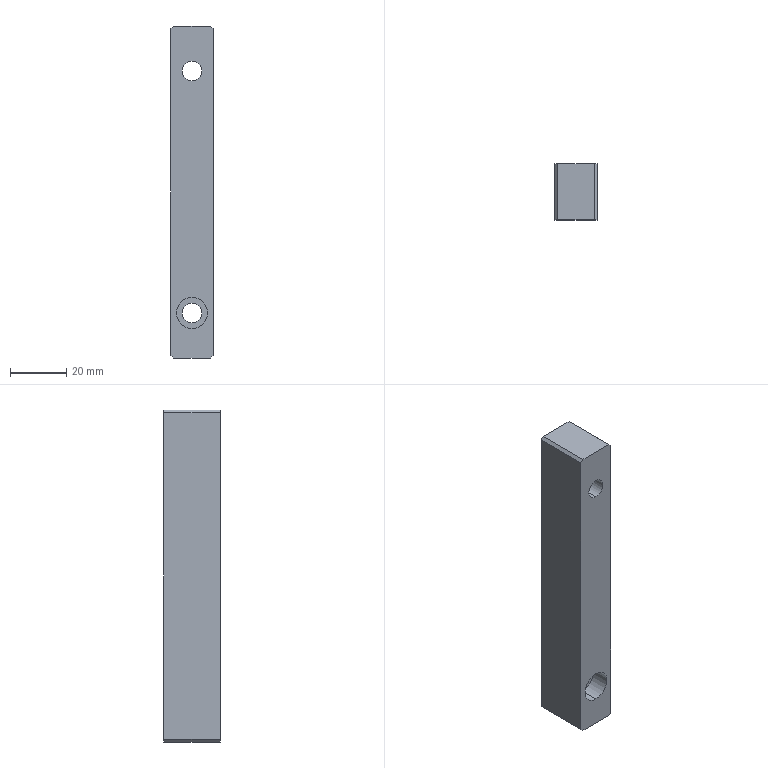Part | NX | features BREP 1 | 1 solid | 20 faces | box 15 x 20 x 118 mm | volume 32871 mm3 | plane 12 | cylinder 8 | commonest cylinder face diameters 7 x4 11 x4
STEP:
#1=CARTESIAN_POINT('',(6.5,20.,0.));
#2=VERTEX_POINT('',#1);
#3=CARTESIAN_POINT('',(7.5,20.,-1.));
#4=VERTEX_POINT('',#3);
#5=CARTESIAN_POINT('',(7.5,20.,-1.));
#6=DIRECTION('',(0.7071,0.,-0.7071));
#7=VECTOR('',#6,1000.);
#8=LINE('',#5,#7);
#9=EDGE_CURVE('',#2,#4,#8,.T.);
#10=ORIENTED_EDGE('',*,*,#9,.F.);
#11=CARTESIAN_POINT('',(6.5,0.,0.));
#12=VERTEX_POINT('',#11);
#13=CARTESIAN_POINT('',(6.5,20.,0.));
#14=DIRECTION('',(0.,1.,0.));
#15=VECTOR('',#14,1000.);
#16=LINE('',#13,#15);
#17=EDGE_CURVE('',#12,#2,#16,.T.);
#18=ORIENTED_EDGE('',*,*,#17,.F.);
#19=CARTESIAN_POINT('',(7.5,0.,-1.));
#20=VERTEX_POINT('',#19);
#21=CARTESIAN_POINT('',(7.5,0.,-1.));
#22=DIRECTION('',(-0.7071,0.,0.7071));
#23=VECTOR('',#22,1000.);
#24=LINE('',#21,#23);
#25=EDGE_CURVE('',#20,#12,#24,.T.);
#26=ORIENTED_EDGE('',*,*,#25,.F.);
#27=CARTESIAN_POINT('',(7.5,0.,-1.));
#28=DIRECTION('',(0.,-1.,0.));
#29=VECTOR('',#28,1000.);
#30=LINE('',#27,#29);
#31=EDGE_CURVE('',#4,#20,#30,.T.);
#32=ORIENTED_EDGE('',*,*,#31,.F.);
#33=EDGE_LOOP('',(#10,#18,#26,#32));
#34=FACE_BOUND('',#33,.T.);
#35=CARTESIAN_POINT('',(7.5,0.,-1.));
#36=DIRECTION('',(0.7071,0.,0.7071));
#37=DIRECTION('',(0.,1.,0.));
#38=AXIS2_PLACEMENT_3D('',#35,#36,#37);
#39=PLANE('',#38);
#40=ADVANCED_FACE('',(#34),#39,.T.);
#41=CARTESIAN_POINT('',(-7.5,20.,-1.));
#42=VERTEX_POINT('',#41);
#43=CARTESIAN_POINT('',(-6.5,20.,0.));
#44=VERTEX_POINT('',#43);
#45=CARTESIAN_POINT('',(-6.5,20.,0.));
#46=DIRECTION('',(0.7071,0.,0.7071));
#47=VECTOR('',#46,1000.);
#48=LINE('',#45,#47);
#49=EDGE_CURVE('',#42,#44,#48,.T.);
#50=ORIENTED_EDGE('',*,*,#49,.F.);
#51=CARTESIAN_POINT('',(-7.5,0.,-1.));
#52=VERTEX_POINT('',#51);
#53=CARTESIAN_POINT('',(-7.5,0.,-1.));
#54=DIRECTION('',(0.,1.,0.));
#55=VECTOR('',#54,1000.);
#56=LINE('',#53,#55);
#57=EDGE_CURVE('',#52,#42,#56,.T.);
#58=ORIENTED_EDGE('',*,*,#57,.F.);
#59=CARTESIAN_POINT('',(-6.5,0.,0.));
#60=VERTEX_POINT('',#59);
#61=CARTESIAN_POINT('',(-6.5,0.,0.));
#62=DIRECTION('',(-0.7071,0.,-0.7071));
#63=VECTOR('',#62,1000.);
#64=LINE('',#61,#63);
#65=EDGE_CURVE('',#60,#52,#64,.T.);
#66=ORIENTED_EDGE('',*,*,#65,.F.);
#67=CARTESIAN_POINT('',(-6.5,20.,0.));
#68=DIRECTION('',(0.,-1.,0.));
#69=VECTOR('',#68,1000.);
#70=LINE('',#67,#69);
#71=EDGE_CURVE('',#44,#60,#70,.T.);
#72=ORIENTED_EDGE('',*,*,#71,.F.);
#73=EDGE_LOOP('',(#50,#58,#66,#72));
#74=FACE_BOUND('',#73,.T.);
#75=CARTESIAN_POINT('',(-6.5,20.,0.));
#76=DIRECTION('',(0.7071,0.,-0.7071));
#77=DIRECTION('',(0.,-1.,0.));
#78=AXIS2_PLACEMENT_3D('',#75,#76,#77);
#79=PLANE('',#78);
#80=ADVANCED_FACE('',(#74),#79,.F.);
#81=CARTESIAN_POINT('',(-7.5,0.,-117.));
#82=VERTEX_POINT('',#81);
#83=CARTESIAN_POINT('',(-6.5,0.,-118.));
#84=VERTEX_POINT('',#83);
#85=CARTESIAN_POINT('',(-6.5,0.,-118.));
#86=DIRECTION('',(0.7071,0.,-0.7071));
#87=VECTOR('',#86,1000.);
#88=LINE('',#85,#87);
#89=EDGE_CURVE('',#82,#84,#88,.T.);
#90=ORIENTED_EDGE('',*,*,#89,.F.);
#91=CARTESIAN_POINT('',(-7.5,20.,-117.));
#92=VERTEX_POINT('',#91);
#93=CARTESIAN_POINT('',(-7.5,0.,-117.));
#94=DIRECTION('',(0.,-1.,0.));
#95=VECTOR('',#94,1000.);
#96=LINE('',#93,#95);
#97=EDGE_CURVE('',#92,#82,#96,.T.);
#98=ORIENTED_EDGE('',*,*,#97,.F.);
#99=CARTESIAN_POINT('',(-6.5,20.,-118.));
#100=VERTEX_POINT('',#99);
#101=CARTESIAN_POINT('',(-6.5,20.,-118.));
#102=DIRECTION('',(-0.7071,0.,0.7071));
#103=VECTOR('',#102,1000.);
#104=LINE('',#101,#103);
#105=EDGE_CURVE('',#100,#92,#104,.T.);
#106=ORIENTED_EDGE('',*,*,#105,.F.);
#107=CARTESIAN_POINT('',(-6.5,20.,-118.));
#108=DIRECTION('',(0.,1.,0.));
#109=VECTOR('',#108,1000.);
#110=LINE('',#107,#109);
#111=EDGE_CURVE('',#84,#100,#110,.T.);
#112=ORIENTED_EDGE('',*,*,#111,.F.);
#113=EDGE_LOOP('',(#90,#98,#106,#112));
#114=FACE_BOUND('',#113,.T.);
#115=CARTESIAN_POINT('',(-6.5,20.,-118.));
#116=DIRECTION('',(0.7071,0.,0.7071));
#117=DIRECTION('',(0.,1.,0.));
#118=AXIS2_PLACEMENT_3D('',#115,#116,#117);
#119=PLANE('',#118);
#120=ADVANCED_FACE('',(#114),#119,.F.);
#121=CARTESIAN_POINT('',(6.5,0.,-118.));
#122=VERTEX_POINT('',#121);
#123=CARTESIAN_POINT('',(7.5,0.,-117.));
#124=VERTEX_POINT('',#123);
#125=CARTESIAN_POINT('',(7.5,0.,-117.));
#126=DIRECTION('',(0.7071,0.,0.7071));
#127=VECTOR('',#126,1000.);
#128=LINE('',#125,#127);
#129=EDGE_CURVE('',#122,#124,#128,.T.);
#130=ORIENTED_EDGE('',*,*,#129,.F.);
#131=CARTESIAN_POINT('',(6.5,20.,-118.));
#132=VERTEX_POINT('',#131);
#133=CARTESIAN_POINT('',(6.5,0.,-118.));
#134=DIRECTION('',(0.,-1.,0.));
#135=VECTOR('',#134,1000.);
#136=LINE('',#133,#135);
#137=EDGE_CURVE('',#132,#122,#136,.T.);
#138=ORIENTED_EDGE('',*,*,#137,.F.);
#139=CARTESIAN_POINT('',(7.5,20.,-117.));
#140=VERTEX_POINT('',#139);
#141=CARTESIAN_POINT('',(7.5,20.,-117.));
#142=DIRECTION('',(-0.7071,0.,-0.7071));
#143=VECTOR('',#142,1000.);
#144=LINE('',#141,#143);
#145=EDGE_CURVE('',#140,#132,#144,.T.);
#146=ORIENTED_EDGE('',*,*,#145,.F.);
#147=CARTESIAN_POINT('',(7.5,20.,-117.));
#148=DIRECTION('',(0.,1.,0.));
#149=VECTOR('',#148,1000.);
#150=LINE('',#147,#149);
#151=EDGE_CURVE('',#124,#140,#150,.T.);
#152=ORIENTED_EDGE('',*,*,#151,.F.);
#153=EDGE_LOOP('',(#130,#138,#146,#152));
#154=FACE_BOUND('',#153,.T.);
#155=CARTESIAN_POINT('',(7.5,0.,-117.));
#156=DIRECTION('',(0.7071,0.,-0.7071));
#157=DIRECTION('',(0.,-1.,0.));
#158=AXIS2_PLACEMENT_3D('',#155,#156,#157);
#159=PLANE('',#158);
#160=ADVANCED_FACE('',(#154),#159,.T.);
#161=CARTESIAN_POINT('',(0.,6.8,-96.5));
#162=VERTEX_POINT('',#161);
#163=CARTESIAN_POINT('',(0.,0.,-96.5));
#164=VERTEX_POINT('',#163);
#165=CARTESIAN_POINT('',(0.,0.,-96.5));
#166=DIRECTION('',(0.,-1.,0.));
#167=VECTOR('',#166,1000.);
#168=LINE('',#165,#167);
#169=EDGE_CURVE('',#162,#164,#168,.T.);
#170=ORIENTED_EDGE('',*,*,#169,.F.);
#171=CARTESIAN_POINT('',(0.,6.8,-107.5));
#172=VERTEX_POINT('',#171);
#173=CARTESIAN_POINT('',(0.,6.8,-102.));
#174=DIRECTION('',(0.,-1.,0.));
#175=DIRECTION('',(0.,0.,-1.));
#176=AXIS2_PLACEMENT_3D('',#173,#174,#175);
#177=CIRCLE('',#176,5.5);
#178=EDGE_CURVE('',#172,#162,#177,.T.);
#179=ORIENTED_EDGE('',*,*,#178,.F.);
#180=CARTESIAN_POINT('',(0.,0.,-107.5));
#181=VERTEX_POINT('',#180);
#182=CARTESIAN_POINT('',(0.,0.,-107.5));
#183=DIRECTION('',(0.,-1.,0.));
#184=VECTOR('',#183,1000.);
#185=LINE('',#182,#184);
#186=EDGE_CURVE('',#172,#181,#185,.T.);
#187=ORIENTED_EDGE('',*,*,#186,.T.);
#188=CARTESIAN_POINT('',(0.,0.,-102.));
#189=DIRECTION('',(0.,-1.,0.));
#190=DIRECTION('',(0.,0.,-1.));
#191=AXIS2_PLACEMENT_3D('',#188,#189,#190);
#192=CIRCLE('',#191,5.5);
#193=EDGE_CURVE('',#181,#164,#192,.T.);
#194=ORIENTED_EDGE('',*,*,#193,.T.);
#195=EDGE_LOOP('',(#170,#179,#187,#194));
#196=FACE_BOUND('',#195,.T.);
#197=CARTESIAN_POINT('',(0.,0.,-102.));
#198=DIRECTION('',(0.,-1.,0.));
#199=DIRECTION('',(0.,0.,-1.));
#200=AXIS2_PLACEMENT_3D('',#197,#198,#199);
#201=CYLINDRICAL_SURFACE('',#200,5.5);
#202=ADVANCED_FACE('',(#196),#201,.F.);
#203=ORIENTED_EDGE('',*,*,#178,.T.);
#204=CARTESIAN_POINT('',(0.,6.8,-102.));
#205=DIRECTION('',(0.,-1.,0.));
#206=DIRECTION('',(0.,0.,-1.));
#207=AXIS2_PLACEMENT_3D('',#204,#205,#206);
#208=CIRCLE('',#207,5.5);
#209=EDGE_CURVE('',#162,#172,#208,.T.);
#210=ORIENTED_EDGE('',*,*,#209,.T.);
#211=EDGE_LOOP('',(#203,#210));
#212=FACE_BOUND('',#211,.T.);
#213=CARTESIAN_POINT('',(0.,6.8,-105.5));
#214=VERTEX_POINT('',#213);
#215=CARTESIAN_POINT('',(0.,6.8,-98.5));
#216=VERTEX_POINT('',#215);
#217=CARTESIAN_POINT('',(0.,6.8,-102.));
#218=DIRECTION('',(0.,-1.,0.));
#219=DIRECTION('',(0.,0.,-1.));
#220=AXIS2_PLACEMENT_3D('',#217,#218,#219);
#221=CIRCLE('',#220,3.5);
#222=EDGE_CURVE('',#214,#216,#221,.T.);
#223=ORIENTED_EDGE('',*,*,#222,.F.);
#224=CARTESIAN_POINT('',(0.,6.8,-102.));
#225=DIRECTION('',(0.,-1.,0.));
#226=DIRECTION('',(0.,0.,-1.));
#227=AXIS2_PLACEMENT_3D('',#224,#225,#226);
#228=CIRCLE('',#227,3.5);
#229=EDGE_CURVE('',#216,#214,#228,.T.);
#230=ORIENTED_EDGE('',*,*,#229,.F.);
#231=EDGE_LOOP('',(#223,#230));
#232=FACE_BOUND('',#231,.T.);
#233=CARTESIAN_POINT('',(3.5,6.8,-102.));
#234=DIRECTION('',(0.,1.,0.));
#235=DIRECTION('',(0.,0.,1.));
#236=AXIS2_PLACEMENT_3D('',#233,#234,#235);
#237=PLANE('',#236);
#238=ADVANCED_FACE('',(#212,#232),#237,.F.);
#239=CARTESIAN_POINT('',(0.,20.,-98.5));
#240=VERTEX_POINT('',#239);
#241=CARTESIAN_POINT('',(0.,0.,-98.5));
#242=DIRECTION('',(0.,-1.,0.));
#243=VECTOR('',#242,1000.);
#244=LINE('',#241,#243);
#245=EDGE_CURVE('',#240,#216,#244,.T.);
#246=ORIENTED_EDGE('',*,*,#245,.F.);
#247=CARTESIAN_POINT('',(0.,20.,-105.5));
#248=VERTEX_POINT('',#247);
#249=CARTESIAN_POINT('',(0.,20.,-102.));
#250=DIRECTION('',(0.,-1.,0.));
#251=DIRECTION('',(0.,0.,-1.));
#252=AXIS2_PLACEMENT_3D('',#249,#250,#251);
#253=CIRCLE('',#252,3.5);
#254=EDGE_CURVE('',#248,#240,#253,.T.);
#255=ORIENTED_EDGE('',*,*,#254,.F.);
#256=CARTESIAN_POINT('',(0.,0.,-105.5));
#257=DIRECTION('',(0.,-1.,0.));
#258=VECTOR('',#257,1000.);
#259=LINE('',#256,#258);
#260=EDGE_CURVE('',#248,#214,#259,.T.);
#261=ORIENTED_EDGE('',*,*,#260,.T.);
#262=ORIENTED_EDGE('',*,*,#222,.T.);
#263=EDGE_LOOP('',(#246,#255,#261,#262));
#264=FACE_BOUND('',#263,.T.);
#265=CARTESIAN_POINT('',(0.,0.,-102.));
#266=DIRECTION('',(0.,-1.,0.));
#267=DIRECTION('',(0.,0.,-1.));
#268=AXIS2_PLACEMENT_3D('',#265,#266,#267);
#269=CYLINDRICAL_SURFACE('',#268,3.5);
#270=ADVANCED_FACE('',(#264),#269,.F.);
#271=CARTESIAN_POINT('',(0.,20.,-21.5));
#272=VERTEX_POINT('',#271);
#273=CARTESIAN_POINT('',(0.,10.,-21.5));
#274=VERTEX_POINT('',#273);
#275=CARTESIAN_POINT('',(0.,20.,-21.5));
#276=DIRECTION('',(0.,1.,0.));
#277=VECTOR('',#276,1000.);
#278=LINE('',#275,#277);
#279=EDGE_CURVE('',#272,#274,#278,.F.);
#280=ORIENTED_EDGE('',*,*,#279,.T.);
#281=CARTESIAN_POINT('',(0.,10.,-10.5));
#282=VERTEX_POINT('',#281);
#283=CARTESIAN_POINT('',(0.,10.,-16.));
#284=DIRECTION('',(0.,1.,0.));
#285=DIRECTION('',(0.,0.,1.));
#286=AXIS2_PLACEMENT_3D('',#283,#284,#285);
#287=CIRCLE('',#286,5.5);
#288=EDGE_CURVE('',#282,#274,#287,.T.);
#289=ORIENTED_EDGE('',*,*,#288,.F.);
#290=CARTESIAN_POINT('',(0.,20.,-10.5));
#291=VERTEX_POINT('',#290);
#292=CARTESIAN_POINT('',(0.,20.,-10.5));
#293=DIRECTION('',(0.,1.,0.));
#294=VECTOR('',#293,1000.);
#295=LINE('',#292,#294);
#296=EDGE_CURVE('',#291,#282,#295,.F.);
#297=ORIENTED_EDGE('',*,*,#296,.F.);
#298=CARTESIAN_POINT('',(0.,20.,-16.));
#299=DIRECTION('',(0.,1.,0.));
#300=DIRECTION('',(0.,0.,1.));
#301=AXIS2_PLACEMENT_3D('',#298,#299,#300);
#302=CIRCLE('',#301,5.5);
#303=EDGE_CURVE('',#291,#272,#302,.T.);
#304=ORIENTED_EDGE('',*,*,#303,.T.);
#305=EDGE_LOOP('',(#280,#289,#297,#304));
#306=FACE_BOUND('',#305,.T.);
#307=CARTESIAN_POINT('',(0.,20.,-16.));
#308=DIRECTION('',(0.,1.,0.));
#309=DIRECTION('',(0.,0.,1.));
#310=AXIS2_PLACEMENT_3D('',#307,#308,#309);
#311=CYLINDRICAL_SURFACE('',#310,5.5);
#312=ADVANCED_FACE('',(#306),#311,.F.);
#313=ORIENTED_EDGE('',*,*,#288,.T.);
#314=CARTESIAN_POINT('',(0.,10.,-16.));
#315=DIRECTION('',(0.,1.,0.));
#316=DIRECTION('',(0.,0.,1.));
#317=AXIS2_PLACEMENT_3D('',#314,#315,#316);
#318=CIRCLE('',#317,5.5);
#319=EDGE_CURVE('',#274,#282,#318,.T.);
#320=ORIENTED_EDGE('',*,*,#319,.T.);
#321=EDGE_LOOP('',(#313,#320));
#322=FACE_BOUND('',#321,.T.);
#323=CARTESIAN_POINT('',(0.,10.,-12.5));
#324=VERTEX_POINT('',#323);
#325=CARTESIAN_POINT('',(0.,10.,-19.5));
#326=VERTEX_POINT('',#325);
#327=CARTESIAN_POINT('',(0.,10.,-16.));
#328=DIRECTION('',(0.,1.,0.));
#329=DIRECTION('',(0.,0.,1.));
#330=AXIS2_PLACEMENT_3D('',#327,#328,#329);
#331=CIRCLE('',#330,3.5);
#332=EDGE_CURVE('',#324,#326,#331,.T.);
#333=ORIENTED_EDGE('',*,*,#332,.F.);
#334=CARTESIAN_POINT('',(0.,10.,-16.));
#335=DIRECTION('',(0.,1.,0.));
#336=DIRECTION('',(0.,0.,1.));
#337=AXIS2_PLACEMENT_3D('',#334,#335,#336);
#338=CIRCLE('',#337,3.5);
#339=EDGE_CURVE('',#326,#324,#338,.T.);
#340=ORIENTED_EDGE('',*,*,#339,.F.);
#341=EDGE_LOOP('',(#333,#340));
#342=FACE_BOUND('',#341,.T.);
#343=CARTESIAN_POINT('',(3.5,10.,-16.));
#344=DIRECTION('',(0.,-1.,0.));
#345=DIRECTION('',(0.,0.,-1.));
#346=AXIS2_PLACEMENT_3D('',#343,#344,#345);
#347=PLANE('',#346);
#348=ADVANCED_FACE('',(#322,#342),#347,.F.);
#349=CARTESIAN_POINT('',(0.,0.,-19.5));
#350=VERTEX_POINT('',#349);
#351=CARTESIAN_POINT('',(0.,20.,-19.5));
#352=DIRECTION('',(0.,1.,0.));
#353=VECTOR('',#352,1000.);
#354=LINE('',#351,#353);
#355=EDGE_CURVE('',#326,#350,#354,.F.);
#356=ORIENTED_EDGE('',*,*,#355,.T.);
#357=CARTESIAN_POINT('',(0.,0.,-12.5));
#358=VERTEX_POINT('',#357);
#359=CARTESIAN_POINT('',(0.,0.,-16.));
#360=DIRECTION('',(0.,1.,0.));
#361=DIRECTION('',(0.,0.,1.));
#362=AXIS2_PLACEMENT_3D('',#359,#360,#361);
#363=CIRCLE('',#362,3.5);
#364=EDGE_CURVE('',#358,#350,#363,.T.);
#365=ORIENTED_EDGE('',*,*,#364,.F.);
#366=CARTESIAN_POINT('',(0.,20.,-12.5));
#367=DIRECTION('',(0.,1.,0.));
#368=VECTOR('',#367,1000.);
#369=LINE('',#366,#368);
#370=EDGE_CURVE('',#324,#358,#369,.F.);
#371=ORIENTED_EDGE('',*,*,#370,.F.);
#372=ORIENTED_EDGE('',*,*,#332,.T.);
#373=EDGE_LOOP('',(#356,#365,#371,#372));
#374=FACE_BOUND('',#373,.T.);
#375=CARTESIAN_POINT('',(0.,20.,-16.));
#376=DIRECTION('',(0.,1.,0.));
#377=DIRECTION('',(0.,0.,1.));
#378=AXIS2_PLACEMENT_3D('',#375,#376,#377);
#379=CYLINDRICAL_SURFACE('',#378,3.5);
#380=ADVANCED_FACE('',(#374),#379,.F.);
#381=CARTESIAN_POINT('',(-7.5,20.,-118.));
#382=DIRECTION('',(0.,0.,1.));
#383=VECTOR('',#382,1000.);
#384=LINE('',#381,#383);
#385=EDGE_CURVE('',#92,#42,#384,.T.);
#386=ORIENTED_EDGE('',*,*,#385,.F.);
#387=ORIENTED_EDGE('',*,*,#97,.T.);
#388=CARTESIAN_POINT('',(-7.5,0.,0.));
#389=DIRECTION('',(0.,0.,-1.));
#390=VECTOR('',#389,1000.);
#391=LINE('',#388,#390);
#392=EDGE_CURVE('',#52,#82,#391,.T.);
#393=ORIENTED_EDGE('',*,*,#392,.F.);
#394=ORIENTED_EDGE('',*,*,#57,.T.);
#395=EDGE_LOOP('',(#386,#387,#393,#394));
#396=FACE_BOUND('',#395,.T.);
#397=CARTESIAN_POINT('',(-7.5,0.,0.));
#398=DIRECTION('',(1.,0.,0.));
#399=DIRECTION('',(0.,0.,-1.));
#400=AXIS2_PLACEMENT_3D('',#397,#398,#399);
#401=PLANE('',#400);
#402=ADVANCED_FACE('',(#396),#401,.F.);
#403=CARTESIAN_POINT('',(7.5,0.,0.));
#404=DIRECTION('',(0.,0.,-1.));
#405=VECTOR('',#404,1000.);
#406=LINE('',#403,#405);
#407=EDGE_CURVE('',#20,#124,#406,.T.);
#408=ORIENTED_EDGE('',*,*,#407,.T.);
#409=ORIENTED_EDGE('',*,*,#151,.T.);
#410=CARTESIAN_POINT('',(7.5,20.,-118.));
#411=DIRECTION('',(0.,0.,1.));
#412=VECTOR('',#411,1000.);
#413=LINE('',#410,#412);
#414=EDGE_CURVE('',#140,#4,#413,.T.);
#415=ORIENTED_EDGE('',*,*,#414,.T.);
#416=ORIENTED_EDGE('',*,*,#31,.T.);
#417=EDGE_LOOP('',(#408,#409,#415,#416));
#418=FACE_BOUND('',#417,.T.);
#419=CARTESIAN_POINT('',(7.5,0.,0.));
#420=DIRECTION('',(1.,0.,0.));
#421=DIRECTION('',(0.,0.,-1.));
#422=AXIS2_PLACEMENT_3D('',#419,#420,#421);
#423=PLANE('',#422);
#424=ADVANCED_FACE('',(#418),#423,.T.);
#425=ORIENTED_EDGE('',*,*,#414,.F.);
#426=ORIENTED_EDGE('',*,*,#145,.T.);
#427=CARTESIAN_POINT('',(7.5,20.,-118.));
#428=DIRECTION('',(-1.,0.,0.));
#429=VECTOR('',#428,1000.);
#430=LINE('',#427,#429);
#431=EDGE_CURVE('',#132,#100,#430,.T.);
#432=ORIENTED_EDGE('',*,*,#431,.T.);
#433=ORIENTED_EDGE('',*,*,#105,.T.);
#434=ORIENTED_EDGE('',*,*,#385,.T.);
#435=ORIENTED_EDGE('',*,*,#49,.T.);
#436=CARTESIAN_POINT('',(7.5,20.,0.));
#437=DIRECTION('',(-1.,0.,0.));
#438=VECTOR('',#437,1000.);
#439=LINE('',#436,#438);
#440=EDGE_CURVE('',#2,#44,#439,.T.);
#441=ORIENTED_EDGE('',*,*,#440,.F.);
#442=ORIENTED_EDGE('',*,*,#9,.T.);
#443=EDGE_LOOP('',(#425,#426,#432,#433,#434,#435,#441,#442));
#444=FACE_BOUND('',#443,.T.);
#445=ORIENTED_EDGE('',*,*,#303,.F.);
#446=CARTESIAN_POINT('',(0.,20.,-16.));
#447=DIRECTION('',(0.,1.,0.));
#448=DIRECTION('',(0.,0.,1.));
#449=AXIS2_PLACEMENT_3D('',#446,#447,#448);
#450=CIRCLE('',#449,5.5);
#451=EDGE_CURVE('',#272,#291,#450,.T.);
#452=ORIENTED_EDGE('',*,*,#451,.F.);
#453=EDGE_LOOP('',(#445,#452));
#454=FACE_BOUND('',#453,.T.);
#455=ORIENTED_EDGE('',*,*,#254,.T.);
#456=CARTESIAN_POINT('',(0.,20.,-102.));
#457=DIRECTION('',(0.,-1.,0.));
#458=DIRECTION('',(0.,0.,-1.));
#459=AXIS2_PLACEMENT_3D('',#456,#457,#458);
#460=CIRCLE('',#459,3.5);
#461=EDGE_CURVE('',#240,#248,#460,.T.);
#462=ORIENTED_EDGE('',*,*,#461,.T.);
#463=EDGE_LOOP('',(#455,#462));
#464=FACE_BOUND('',#463,.T.);
#465=CARTESIAN_POINT('',(7.5,20.,-118.));
#466=DIRECTION('',(0.,-1.,0.));
#467=DIRECTION('',(0.,0.,-1.));
#468=AXIS2_PLACEMENT_3D('',#465,#466,#467);
#469=PLANE('',#468);
#470=ADVANCED_FACE('',(#444,#454,#464),#469,.F.);
#471=ORIENTED_EDGE('',*,*,#431,.F.);
#472=ORIENTED_EDGE('',*,*,#137,.T.);
#473=CARTESIAN_POINT('',(7.5,0.,-118.));
#474=DIRECTION('',(-1.,0.,0.));
#475=VECTOR('',#474,1000.);
#476=LINE('',#473,#475);
#477=EDGE_CURVE('',#122,#84,#476,.T.);
#478=ORIENTED_EDGE('',*,*,#477,.T.);
#479=ORIENTED_EDGE('',*,*,#111,.T.);
#480=EDGE_LOOP('',(#471,#472,#478,#479));
#481=FACE_BOUND('',#480,.T.);
#482=CARTESIAN_POINT('',(7.5,20.,-118.));
#483=DIRECTION('',(0.,0.,1.));
#484=DIRECTION('',(1.,0.,0.));
#485=AXIS2_PLACEMENT_3D('',#482,#483,#484);
#486=PLANE('',#485);
#487=ADVANCED_FACE('',(#481),#486,.F.);
#488=ORIENTED_EDGE('',*,*,#477,.F.);
#489=ORIENTED_EDGE('',*,*,#129,.T.);
#490=ORIENTED_EDGE('',*,*,#407,.F.);
#491=ORIENTED_EDGE('',*,*,#25,.T.);
#492=CARTESIAN_POINT('',(7.5,0.,0.));
#493=DIRECTION('',(-1.,0.,0.));
#494=VECTOR('',#493,1000.);
#495=LINE('',#492,#494);
#496=EDGE_CURVE('',#12,#60,#495,.T.);
#497=ORIENTED_EDGE('',*,*,#496,.T.);
#498=ORIENTED_EDGE('',*,*,#65,.T.);
#499=ORIENTED_EDGE('',*,*,#392,.T.);
#500=ORIENTED_EDGE('',*,*,#89,.T.);
#501=EDGE_LOOP('',(#488,#489,#490,#491,#497,#498,#499,#500));
#502=FACE_BOUND('',#501,.T.);
#503=ORIENTED_EDGE('',*,*,#364,.T.);
#504=CARTESIAN_POINT('',(0.,0.,-16.));
#505=DIRECTION('',(0.,1.,0.));
#506=DIRECTION('',(0.,0.,1.));
#507=AXIS2_PLACEMENT_3D('',#504,#505,#506);
#508=CIRCLE('',#507,3.5);
#509=EDGE_CURVE('',#350,#358,#508,.T.);
#510=ORIENTED_EDGE('',*,*,#509,.T.);
#511=EDGE_LOOP('',(#503,#510));
#512=FACE_BOUND('',#511,.T.);
#513=ORIENTED_EDGE('',*,*,#193,.F.);
#514=CARTESIAN_POINT('',(0.,0.,-102.));
#515=DIRECTION('',(0.,-1.,0.));
#516=DIRECTION('',(0.,0.,-1.));
#517=AXIS2_PLACEMENT_3D('',#514,#515,#516);
#518=CIRCLE('',#517,5.5);
#519=EDGE_CURVE('',#164,#181,#518,.T.);
#520=ORIENTED_EDGE('',*,*,#519,.F.);
#521=EDGE_LOOP('',(#513,#520));
#522=FACE_BOUND('',#521,.T.);
#523=CARTESIAN_POINT('',(7.5,0.,0.));
#524=DIRECTION('',(0.,1.,0.));
#525=DIRECTION('',(0.,0.,1.));
#526=AXIS2_PLACEMENT_3D('',#523,#524,#525);
#527=PLANE('',#526);
#528=ADVANCED_FACE('',(#502,#512,#522),#527,.F.);
#529=ORIENTED_EDGE('',*,*,#440,.T.);
#530=ORIENTED_EDGE('',*,*,#71,.T.);
#531=ORIENTED_EDGE('',*,*,#496,.F.);
#532=ORIENTED_EDGE('',*,*,#17,.T.);
#533=EDGE_LOOP('',(#529,#530,#531,#532));
#534=FACE_BOUND('',#533,.T.);
#535=CARTESIAN_POINT('',(7.5,20.,0.));
#536=DIRECTION('',(0.,0.,-1.));
#537=DIRECTION('',(0.,1.,0.));
#538=AXIS2_PLACEMENT_3D('',#535,#536,#537);
#539=PLANE('',#538);
#540=ADVANCED_FACE('',(#534),#539,.F.);
#541=ORIENTED_EDGE('',*,*,#509,.F.);
#542=ORIENTED_EDGE('',*,*,#355,.F.);
#543=ORIENTED_EDGE('',*,*,#339,.T.);
#544=ORIENTED_EDGE('',*,*,#370,.T.);
#545=EDGE_LOOP('',(#541,#542,#543,#544));
#546=FACE_BOUND('',#545,.T.);
#547=CARTESIAN_POINT('',(0.,20.,-16.));
#548=DIRECTION('',(0.,1.,0.));
#549=DIRECTION('',(0.,0.,1.));
#550=AXIS2_PLACEMENT_3D('',#547,#548,#549);
#551=CYLINDRICAL_SURFACE('',#550,3.5);
#552=ADVANCED_FACE('',(#546),#551,.F.);
#553=ORIENTED_EDGE('',*,*,#319,.F.);
#554=ORIENTED_EDGE('',*,*,#279,.F.);
#555=ORIENTED_EDGE('',*,*,#451,.T.);
#556=ORIENTED_EDGE('',*,*,#296,.T.);
#557=EDGE_LOOP('',(#553,#554,#555,#556));
#558=FACE_BOUND('',#557,.T.);
#559=CARTESIAN_POINT('',(0.,20.,-16.));
#560=DIRECTION('',(0.,1.,0.));
#561=DIRECTION('',(0.,0.,1.));
#562=AXIS2_PLACEMENT_3D('',#559,#560,#561);
#563=CYLINDRICAL_SURFACE('',#562,5.5);
#564=ADVANCED_FACE('',(#558),#563,.F.);
#565=ORIENTED_EDGE('',*,*,#461,.F.);
#566=ORIENTED_EDGE('',*,*,#245,.T.);
#567=ORIENTED_EDGE('',*,*,#229,.T.);
#568=ORIENTED_EDGE('',*,*,#260,.F.);
#569=EDGE_LOOP('',(#565,#566,#567,#568));
#570=FACE_BOUND('',#569,.T.);
#571=CARTESIAN_POINT('',(0.,0.,-102.));
#572=DIRECTION('',(0.,-1.,0.));
#573=DIRECTION('',(0.,0.,-1.));
#574=AXIS2_PLACEMENT_3D('',#571,#572,#573);
#575=CYLINDRICAL_SURFACE('',#574,3.5);
#576=ADVANCED_FACE('',(#570),#575,.F.);
#577=ORIENTED_EDGE('',*,*,#209,.F.);
#578=ORIENTED_EDGE('',*,*,#169,.T.);
#579=ORIENTED_EDGE('',*,*,#519,.T.);
#580=ORIENTED_EDGE('',*,*,#186,.F.);
#581=EDGE_LOOP('',(#577,#578,#579,#580));
#582=FACE_BOUND('',#581,.T.);
#583=CARTESIAN_POINT('',(0.,0.,-102.));
#584=DIRECTION('',(0.,-1.,0.));
#585=DIRECTION('',(0.,0.,-1.));
#586=AXIS2_PLACEMENT_3D('',#583,#584,#585);
#587=CYLINDRICAL_SURFACE('',#586,5.5);
#588=ADVANCED_FACE('',(#582),#587,.F.);
#589=CLOSED_SHELL('',(#40,#80,#120,#160,#202,#238,#270,#312,#348,#380,#402,#424,#470,#487,#528,#540,#552,#564,#576,#588));
#590=MANIFOLD_SOLID_BREP('',#589);
#591=(LENGTH_UNIT()NAMED_UNIT(*)SI_UNIT(.MILLI.,.METRE.));
#592=UNCERTAINTY_MEASURE_WITH_UNIT(LENGTH_MEASURE(0.00001),#591,'','');
#593=(NAMED_UNIT(*)PLANE_ANGLE_UNIT()SI_UNIT($,.RADIAN.));
#594=(NAMED_UNIT(*)SI_UNIT($,.STERADIAN.)SOLID_ANGLE_UNIT());
#595=(GEOMETRIC_REPRESENTATION_CONTEXT(3)GLOBAL_UNCERTAINTY_ASSIGNED_CONTEXT((#592))GLOBAL_UNIT_ASSIGNED_CONTEXT((#591,#593,#594))REPRESENTATION_CONTEXT('',''));
#596=ADVANCED_BREP_SHAPE_REPRESENTATION('',(#590),#595);